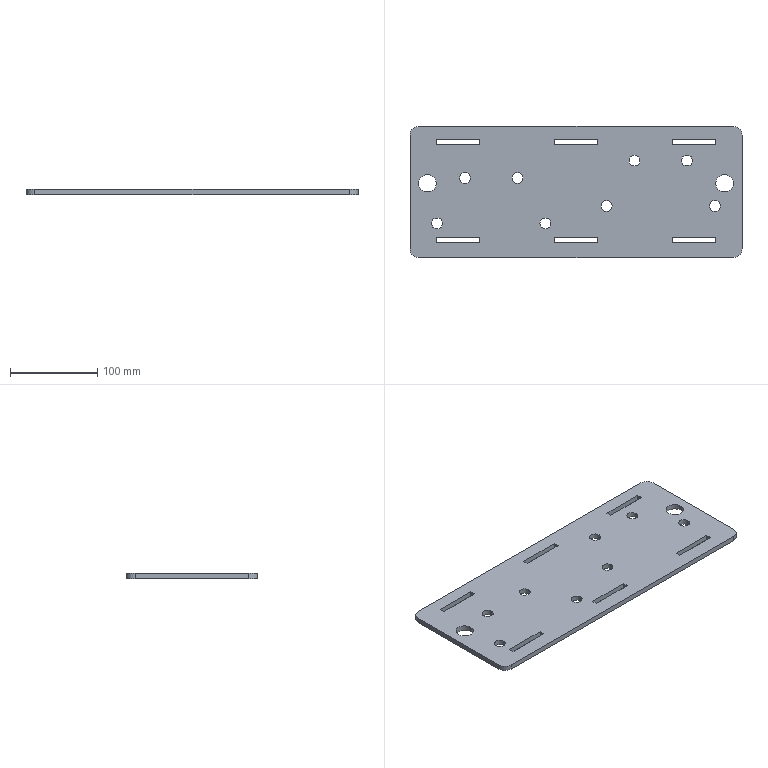Part | SolidWorks | features FlatPattern 1, SMBaseFlange 1, SheetMetal 1 | 1 solid | 54 faces | box 380 x 150 x 6 mm | volume 321025 mm3 | plane 30 | cylinder 24 | commonest cylinder face diameters 12.5 x16 20 x8